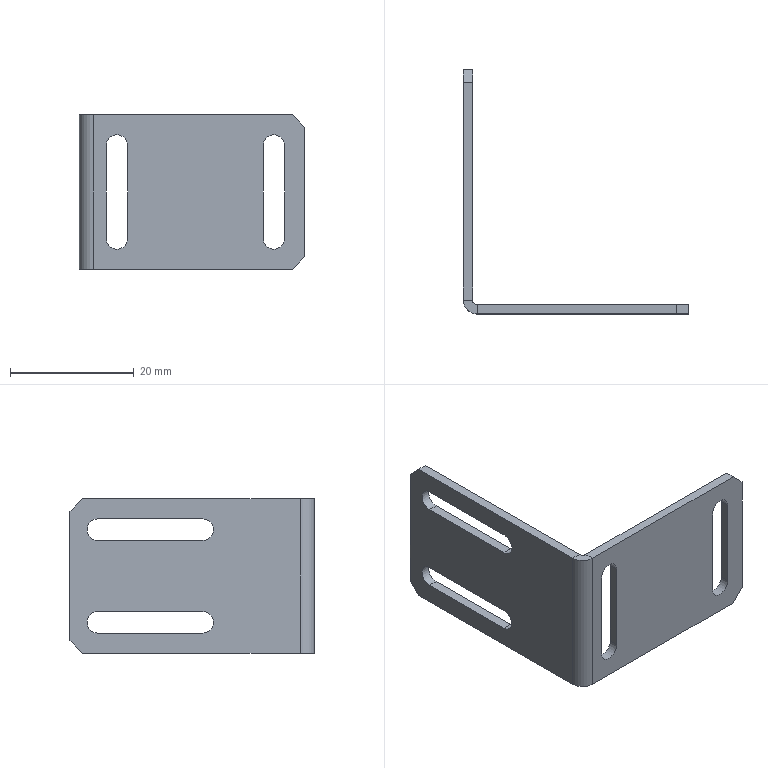Part | NX | 1 solid | 34 faces | box 36.5 x 39.5 x 25 mm | volume 2364 mm3 | plane 24 | cylinder 10 | commonest cylinder face diameters 3.5 x8 1.473 x1 4.473 x1
STEP:
#1=CARTESIAN_POINT('',(-1.5,-18.263,-12.5));
#2=VERTEX_POINT('',#1);
#3=CARTESIAN_POINT('',(-1.5,17.,-12.5));
#4=VERTEX_POINT('',#3);
#5=CARTESIAN_POINT('',(-1.5,-19.,-12.5));
#6=DIRECTION('',(0.,1.,0.));
#7=VECTOR('',#6,1000.);
#8=LINE('',#5,#7);
#9=EDGE_CURVE('',#2,#4,#8,.T.);
#10=ORIENTED_EDGE('',*,*,#9,.T.);
#11=CARTESIAN_POINT('',(0.,17.,-12.5));
#12=VERTEX_POINT('',#11);
#13=CARTESIAN_POINT('',(-1.5,17.,-12.5));
#14=DIRECTION('',(1.,0.,0.));
#15=VECTOR('',#14,1000.);
#16=LINE('',#13,#15);
#17=EDGE_CURVE('',#4,#12,#16,.T.);
#18=ORIENTED_EDGE('',*,*,#17,.T.);
#19=CARTESIAN_POINT('',(0.,-18.263,-12.5));
#20=VERTEX_POINT('',#19);
#21=CARTESIAN_POINT('',(0.,-19.,-12.5));
#22=DIRECTION('',(0.,1.,0.));
#23=VECTOR('',#22,1000.);
#24=LINE('',#21,#23);
#25=EDGE_CURVE('',#20,#12,#24,.T.);
#26=ORIENTED_EDGE('',*,*,#25,.F.);
#27=CARTESIAN_POINT('',(0.,-18.263,-12.5));
#28=DIRECTION('',(-1.,0.,0.));
#29=VECTOR('',#28,1000.);
#30=LINE('',#27,#29);
#31=EDGE_CURVE('',#20,#2,#30,.T.);
#32=ORIENTED_EDGE('',*,*,#31,.T.);
#33=EDGE_LOOP('',(#10,#18,#26,#32));
#34=FACE_BOUND('',#33,.T.);
#35=CARTESIAN_POINT('',(-1.5,-19.,-12.5));
#36=DIRECTION('',(0.,0.,-1.));
#37=DIRECTION('',(-1.,0.,0.));
#38=AXIS2_PLACEMENT_3D('',#35,#36,#37);
#39=PLANE('',#38);
#40=ADVANCED_FACE('',(#34),#39,.T.);
#41=CARTESIAN_POINT('',(-1.5,14.5,-9.25));
#42=VERTEX_POINT('',#41);
#43=CARTESIAN_POINT('',(-1.5,14.5,-5.75));
#44=VERTEX_POINT('',#43);
#45=CARTESIAN_POINT('',(-1.5,14.5,-7.5));
#46=DIRECTION('',(1.,0.,0.));
#47=DIRECTION('',(0.,0.,-1.));
#48=AXIS2_PLACEMENT_3D('',#45,#46,#47);
#49=CIRCLE('',#48,1.75);
#50=EDGE_CURVE('',#42,#44,#49,.T.);
#51=ORIENTED_EDGE('',*,*,#50,.T.);
#52=CARTESIAN_POINT('',(-1.5,-2.5,-5.75));
#53=VERTEX_POINT('',#52);
#54=CARTESIAN_POINT('',(-1.5,14.5,-5.75));
#55=DIRECTION('',(0.,-1.,0.));
#56=VECTOR('',#55,1000.);
#57=LINE('',#54,#56);
#58=EDGE_CURVE('',#44,#53,#57,.T.);
#59=ORIENTED_EDGE('',*,*,#58,.T.);
#60=CARTESIAN_POINT('',(-1.5,-2.5,-9.25));
#61=VERTEX_POINT('',#60);
#62=CARTESIAN_POINT('',(-1.5,-2.5,-7.5));
#63=DIRECTION('',(1.,0.,0.));
#64=DIRECTION('',(0.,0.,-1.));
#65=AXIS2_PLACEMENT_3D('',#62,#63,#64);
#66=CIRCLE('',#65,1.75);
#67=EDGE_CURVE('',#53,#61,#66,.T.);
#68=ORIENTED_EDGE('',*,*,#67,.T.);
#69=CARTESIAN_POINT('',(-1.5,14.5,-9.25));
#70=DIRECTION('',(0.,1.,0.));
#71=VECTOR('',#70,1000.);
#72=LINE('',#69,#71);
#73=EDGE_CURVE('',#61,#42,#72,.T.);
#74=ORIENTED_EDGE('',*,*,#73,.T.);
#75=EDGE_LOOP('',(#51,#59,#68,#74));
#76=FACE_BOUND('',#75,.T.);
#77=CARTESIAN_POINT('',(-1.5,14.5,5.75));
#78=VERTEX_POINT('',#77);
#79=CARTESIAN_POINT('',(-1.5,14.5,9.25));
#80=VERTEX_POINT('',#79);
#81=CARTESIAN_POINT('',(-1.5,14.5,7.5));
#82=DIRECTION('',(1.,0.,0.));
#83=DIRECTION('',(0.,0.,-1.));
#84=AXIS2_PLACEMENT_3D('',#81,#82,#83);
#85=CIRCLE('',#84,1.75);
#86=EDGE_CURVE('',#78,#80,#85,.T.);
#87=ORIENTED_EDGE('',*,*,#86,.T.);
#88=CARTESIAN_POINT('',(-1.5,-2.5,9.25));
#89=VERTEX_POINT('',#88);
#90=CARTESIAN_POINT('',(-1.5,14.5,9.25));
#91=DIRECTION('',(0.,-1.,0.));
#92=VECTOR('',#91,1000.);
#93=LINE('',#90,#92);
#94=EDGE_CURVE('',#80,#89,#93,.T.);
#95=ORIENTED_EDGE('',*,*,#94,.T.);
#96=CARTESIAN_POINT('',(-1.5,-2.5,5.75));
#97=VERTEX_POINT('',#96);
#98=CARTESIAN_POINT('',(-1.5,-2.5,7.5));
#99=DIRECTION('',(1.,0.,0.));
#100=DIRECTION('',(0.,0.,-1.));
#101=AXIS2_PLACEMENT_3D('',#98,#99,#100);
#102=CIRCLE('',#101,1.75);
#103=EDGE_CURVE('',#89,#97,#102,.T.);
#104=ORIENTED_EDGE('',*,*,#103,.T.);
#105=CARTESIAN_POINT('',(-1.5,14.5,5.75));
#106=DIRECTION('',(0.,1.,0.));
#107=VECTOR('',#106,1000.);
#108=LINE('',#105,#107);
#109=EDGE_CURVE('',#97,#78,#108,.T.);
#110=ORIENTED_EDGE('',*,*,#109,.T.);
#111=EDGE_LOOP('',(#87,#95,#104,#110));
#112=FACE_BOUND('',#111,.T.);
#113=CARTESIAN_POINT('',(-1.5,19.,-10.5));
#114=VERTEX_POINT('',#113);
#115=CARTESIAN_POINT('',(-1.5,19.,10.5));
#116=VERTEX_POINT('',#115);
#117=CARTESIAN_POINT('',(-1.5,19.,12.5));
#118=DIRECTION('',(0.,0.,1.));
#119=VECTOR('',#118,1000.);
#120=LINE('',#117,#119);
#121=EDGE_CURVE('',#114,#116,#120,.T.);
#122=ORIENTED_EDGE('',*,*,#121,.F.);
#123=CARTESIAN_POINT('',(-1.5,14.75,-14.75));
#124=DIRECTION('',(0.,0.7071,0.7071));
#125=VECTOR('',#124,1000.);
#126=LINE('',#123,#125);
#127=EDGE_CURVE('',#114,#4,#126,.F.);
#128=ORIENTED_EDGE('',*,*,#127,.T.);
#129=ORIENTED_EDGE('',*,*,#9,.F.);
#130=CARTESIAN_POINT('',(-1.5,-18.263,12.5));
#131=VERTEX_POINT('',#130);
#132=CARTESIAN_POINT('',(-1.5,-18.263,-12.5));
#133=DIRECTION('',(0.,0.,-1.));
#134=VECTOR('',#133,1000.);
#135=LINE('',#132,#134);
#136=EDGE_CURVE('',#2,#131,#135,.F.);
#137=ORIENTED_EDGE('',*,*,#136,.T.);
#138=CARTESIAN_POINT('',(-1.5,17.,12.5));
#139=VERTEX_POINT('',#138);
#140=CARTESIAN_POINT('',(-1.5,-19.,12.5));
#141=DIRECTION('',(0.,-1.,0.));
#142=VECTOR('',#141,1000.);
#143=LINE('',#140,#142);
#144=EDGE_CURVE('',#139,#131,#143,.T.);
#145=ORIENTED_EDGE('',*,*,#144,.F.);
#146=CARTESIAN_POINT('',(-1.5,14.75,14.75));
#147=DIRECTION('',(0.,-0.7071,0.7071));
#148=VECTOR('',#147,1000.);
#149=LINE('',#146,#148);
#150=EDGE_CURVE('',#139,#116,#149,.F.);
#151=ORIENTED_EDGE('',*,*,#150,.T.);
#152=EDGE_LOOP('',(#122,#128,#129,#137,#145,#151));
#153=FACE_BOUND('',#152,.T.);
#154=CARTESIAN_POINT('',(-1.5,0.,0.));
#155=DIRECTION('',(-1.,0.,0.));
#156=DIRECTION('',(0.,0.,1.));
#157=AXIS2_PLACEMENT_3D('',#154,#155,#156);
#158=PLANE('',#157);
#159=ADVANCED_FACE('',(#76,#112,#153),#158,.T.);
#160=CARTESIAN_POINT('',(0.,14.5,-5.75));
#161=VERTEX_POINT('',#160);
#162=CARTESIAN_POINT('',(0.,-2.5,-5.75));
#163=VERTEX_POINT('',#162);
#164=CARTESIAN_POINT('',(0.,14.5,-5.75));
#165=DIRECTION('',(0.,-1.,0.));
#166=VECTOR('',#165,1000.);
#167=LINE('',#164,#166);
#168=EDGE_CURVE('',#161,#163,#167,.T.);
#169=ORIENTED_EDGE('',*,*,#168,.F.);
#170=CARTESIAN_POINT('',(0.,14.5,-9.25));
#171=VERTEX_POINT('',#170);
#172=CARTESIAN_POINT('',(0.,14.5,-7.5));
#173=DIRECTION('',(1.,0.,0.));
#174=DIRECTION('',(0.,0.,-1.));
#175=AXIS2_PLACEMENT_3D('',#172,#173,#174);
#176=CIRCLE('',#175,1.75);
#177=EDGE_CURVE('',#171,#161,#176,.T.);
#178=ORIENTED_EDGE('',*,*,#177,.F.);
#179=CARTESIAN_POINT('',(0.,-2.5,-9.25));
#180=VERTEX_POINT('',#179);
#181=CARTESIAN_POINT('',(0.,14.5,-9.25));
#182=DIRECTION('',(0.,1.,0.));
#183=VECTOR('',#182,1000.);
#184=LINE('',#181,#183);
#185=EDGE_CURVE('',#180,#171,#184,.T.);
#186=ORIENTED_EDGE('',*,*,#185,.F.);
#187=CARTESIAN_POINT('',(0.,-2.5,-7.5));
#188=DIRECTION('',(1.,0.,0.));
#189=DIRECTION('',(0.,0.,-1.));
#190=AXIS2_PLACEMENT_3D('',#187,#188,#189);
#191=CIRCLE('',#190,1.75);
#192=EDGE_CURVE('',#163,#180,#191,.T.);
#193=ORIENTED_EDGE('',*,*,#192,.F.);
#194=EDGE_LOOP('',(#169,#178,#186,#193));
#195=FACE_BOUND('',#194,.T.);
#196=CARTESIAN_POINT('',(0.,14.5,9.25));
#197=VERTEX_POINT('',#196);
#198=CARTESIAN_POINT('',(0.,-2.5,9.25));
#199=VERTEX_POINT('',#198);
#200=CARTESIAN_POINT('',(0.,14.5,9.25));
#201=DIRECTION('',(0.,-1.,0.));
#202=VECTOR('',#201,1000.);
#203=LINE('',#200,#202);
#204=EDGE_CURVE('',#197,#199,#203,.T.);
#205=ORIENTED_EDGE('',*,*,#204,.F.);
#206=CARTESIAN_POINT('',(0.,14.5,5.75));
#207=VERTEX_POINT('',#206);
#208=CARTESIAN_POINT('',(0.,14.5,7.5));
#209=DIRECTION('',(1.,0.,0.));
#210=DIRECTION('',(0.,0.,-1.));
#211=AXIS2_PLACEMENT_3D('',#208,#209,#210);
#212=CIRCLE('',#211,1.75);
#213=EDGE_CURVE('',#207,#197,#212,.T.);
#214=ORIENTED_EDGE('',*,*,#213,.F.);
#215=CARTESIAN_POINT('',(0.,-2.5,5.75));
#216=VERTEX_POINT('',#215);
#217=CARTESIAN_POINT('',(0.,14.5,5.75));
#218=DIRECTION('',(0.,1.,0.));
#219=VECTOR('',#218,1000.);
#220=LINE('',#217,#219);
#221=EDGE_CURVE('',#216,#207,#220,.T.);
#222=ORIENTED_EDGE('',*,*,#221,.F.);
#223=CARTESIAN_POINT('',(0.,-2.5,7.5));
#224=DIRECTION('',(1.,0.,0.));
#225=DIRECTION('',(0.,0.,-1.));
#226=AXIS2_PLACEMENT_3D('',#223,#224,#225);
#227=CIRCLE('',#226,1.75);
#228=EDGE_CURVE('',#199,#216,#227,.T.);
#229=ORIENTED_EDGE('',*,*,#228,.F.);
#230=EDGE_LOOP('',(#205,#214,#222,#229));
#231=FACE_BOUND('',#230,.T.);
#232=ORIENTED_EDGE('',*,*,#25,.T.);
#233=CARTESIAN_POINT('',(0.,19.,-10.5));
#234=VERTEX_POINT('',#233);
#235=CARTESIAN_POINT('',(0.,17.,-12.5));
#236=DIRECTION('',(0.,-0.7071,-0.7071));
#237=VECTOR('',#236,1000.);
#238=LINE('',#235,#237);
#239=EDGE_CURVE('',#12,#234,#238,.F.);
#240=ORIENTED_EDGE('',*,*,#239,.T.);
#241=CARTESIAN_POINT('',(0.,19.,10.5));
#242=VERTEX_POINT('',#241);
#243=CARTESIAN_POINT('',(0.,19.,12.5));
#244=DIRECTION('',(0.,0.,1.));
#245=VECTOR('',#244,1000.);
#246=LINE('',#243,#245);
#247=EDGE_CURVE('',#234,#242,#246,.T.);
#248=ORIENTED_EDGE('',*,*,#247,.T.);
#249=CARTESIAN_POINT('',(0.,17.,12.5));
#250=VERTEX_POINT('',#249);
#251=CARTESIAN_POINT('',(0.,19.,10.5));
#252=DIRECTION('',(0.,0.7071,-0.7071));
#253=VECTOR('',#252,1000.);
#254=LINE('',#251,#253);
#255=EDGE_CURVE('',#242,#250,#254,.F.);
#256=ORIENTED_EDGE('',*,*,#255,.T.);
#257=CARTESIAN_POINT('',(0.,-18.263,12.5));
#258=VERTEX_POINT('',#257);
#259=CARTESIAN_POINT('',(0.,-19.,12.5));
#260=DIRECTION('',(0.,-1.,0.));
#261=VECTOR('',#260,1000.);
#262=LINE('',#259,#261);
#263=EDGE_CURVE('',#250,#258,#262,.T.);
#264=ORIENTED_EDGE('',*,*,#263,.T.);
#265=CARTESIAN_POINT('',(0.,-18.263,-12.5));
#266=DIRECTION('',(0.,0.,-1.));
#267=VECTOR('',#266,1000.);
#268=LINE('',#265,#267);
#269=EDGE_CURVE('',#20,#258,#268,.F.);
#270=ORIENTED_EDGE('',*,*,#269,.F.);
#271=EDGE_LOOP('',(#232,#240,#248,#256,#264,#270));
#272=FACE_BOUND('',#271,.T.);
#273=CARTESIAN_POINT('',(0.,0.,0.));
#274=DIRECTION('',(-1.,0.,0.));
#275=DIRECTION('',(0.,0.,1.));
#276=AXIS2_PLACEMENT_3D('',#273,#274,#275);
#277=PLANE('',#276);
#278=ADVANCED_FACE('',(#195,#231,#272),#277,.F.);
#279=ORIENTED_EDGE('',*,*,#263,.F.);
#280=CARTESIAN_POINT('',(-1.5,17.,12.5));
#281=DIRECTION('',(-1.,0.,0.));
#282=VECTOR('',#281,1000.);
#283=LINE('',#280,#282);
#284=EDGE_CURVE('',#250,#139,#283,.T.);
#285=ORIENTED_EDGE('',*,*,#284,.T.);
#286=ORIENTED_EDGE('',*,*,#144,.T.);
#287=CARTESIAN_POINT('',(0.,-18.263,12.5));
#288=DIRECTION('',(-1.,0.,0.));
#289=VECTOR('',#288,1000.);
#290=LINE('',#287,#289);
#291=EDGE_CURVE('',#258,#131,#290,.T.);
#292=ORIENTED_EDGE('',*,*,#291,.F.);
#293=EDGE_LOOP('',(#279,#285,#286,#292));
#294=FACE_BOUND('',#293,.T.);
#295=CARTESIAN_POINT('',(-1.5,-19.,12.5));
#296=DIRECTION('',(0.,0.,1.));
#297=DIRECTION('',(1.,0.,0.));
#298=AXIS2_PLACEMENT_3D('',#295,#296,#297);
#299=PLANE('',#298);
#300=ADVANCED_FACE('',(#294),#299,.T.);
#301=ORIENTED_EDGE('',*,*,#247,.F.);
#302=CARTESIAN_POINT('',(-1.5,19.,-10.5));
#303=DIRECTION('',(-1.,0.,0.));
#304=VECTOR('',#303,1000.);
#305=LINE('',#302,#304);
#306=EDGE_CURVE('',#234,#114,#305,.T.);
#307=ORIENTED_EDGE('',*,*,#306,.T.);
#308=ORIENTED_EDGE('',*,*,#121,.T.);
#309=CARTESIAN_POINT('',(-1.5,19.,10.5));
#310=DIRECTION('',(1.,0.,0.));
#311=VECTOR('',#310,1000.);
#312=LINE('',#309,#311);
#313=EDGE_CURVE('',#116,#242,#312,.T.);
#314=ORIENTED_EDGE('',*,*,#313,.T.);
#315=EDGE_LOOP('',(#301,#307,#308,#314));
#316=FACE_BOUND('',#315,.T.);
#317=CARTESIAN_POINT('',(-1.5,19.,12.5));
#318=DIRECTION('',(0.,1.,0.));
#319=DIRECTION('',(0.,0.,1.));
#320=AXIS2_PLACEMENT_3D('',#317,#318,#319);
#321=PLANE('',#320);
#322=ADVANCED_FACE('',(#316),#321,.T.);
#323=CARTESIAN_POINT('',(0.7366,-19.,12.5));
#324=VERTEX_POINT('',#323);
#325=CARTESIAN_POINT('',(0.7366,-20.5,12.5));
#326=VERTEX_POINT('',#325);
#327=CARTESIAN_POINT('',(0.7366,-19.,12.5));
#328=DIRECTION('',(0.,-1.,0.));
#329=VECTOR('',#328,1000.);
#330=LINE('',#327,#329);
#331=EDGE_CURVE('',#324,#326,#330,.T.);
#332=ORIENTED_EDGE('',*,*,#331,.F.);
#333=CARTESIAN_POINT('',(0.7366,-18.263,12.5));
#334=DIRECTION('',(0.,0.,-1.));
#335=DIRECTION('',(-1.,0.,0.));
#336=AXIS2_PLACEMENT_3D('',#333,#334,#335);
#337=CIRCLE('',#336,0.7366);
#338=EDGE_CURVE('',#258,#324,#337,.F.);
#339=ORIENTED_EDGE('',*,*,#338,.F.);
#340=ORIENTED_EDGE('',*,*,#291,.T.);
#341=CARTESIAN_POINT('',(0.7366,-18.263,12.5));
#342=DIRECTION('',(0.,0.,-1.));
#343=DIRECTION('',(-1.,0.,0.));
#344=AXIS2_PLACEMENT_3D('',#341,#342,#343);
#345=CIRCLE('',#344,2.237);
#346=EDGE_CURVE('',#131,#326,#345,.F.);
#347=ORIENTED_EDGE('',*,*,#346,.T.);
#348=EDGE_LOOP('',(#332,#339,#340,#347));
#349=FACE_BOUND('',#348,.T.);
#350=CARTESIAN_POINT('',(0.7366,-18.263,12.5));
#351=DIRECTION('',(0.,0.,1.));
#352=DIRECTION('',(1.,0.,0.));
#353=AXIS2_PLACEMENT_3D('',#350,#351,#352);
#354=PLANE('',#353);
#355=ADVANCED_FACE('',(#349),#354,.T.);
#356=CARTESIAN_POINT('',(0.7366,-19.,-12.5));
#357=VERTEX_POINT('',#356);
#358=CARTESIAN_POINT('',(0.7366,-18.263,-12.5));
#359=DIRECTION('',(0.,0.,-1.));
#360=DIRECTION('',(-1.,0.,0.));
#361=AXIS2_PLACEMENT_3D('',#358,#359,#360);
#362=CIRCLE('',#361,0.7366);
#363=EDGE_CURVE('',#357,#20,#362,.T.);
#364=ORIENTED_EDGE('',*,*,#363,.F.);
#365=CARTESIAN_POINT('',(0.7366,-20.5,-12.5));
#366=VERTEX_POINT('',#365);
#367=CARTESIAN_POINT('',(0.7366,-19.,-12.5));
#368=DIRECTION('',(0.,-1.,0.));
#369=VECTOR('',#368,1000.);
#370=LINE('',#367,#369);
#371=EDGE_CURVE('',#357,#366,#370,.T.);
#372=ORIENTED_EDGE('',*,*,#371,.T.);
#373=CARTESIAN_POINT('',(0.7366,-18.263,-12.5));
#374=DIRECTION('',(0.,0.,-1.));
#375=DIRECTION('',(-1.,0.,0.));
#376=AXIS2_PLACEMENT_3D('',#373,#374,#375);
#377=CIRCLE('',#376,2.237);
#378=EDGE_CURVE('',#366,#2,#377,.T.);
#379=ORIENTED_EDGE('',*,*,#378,.T.);
#380=ORIENTED_EDGE('',*,*,#31,.F.);
#381=EDGE_LOOP('',(#364,#372,#379,#380));
#382=FACE_BOUND('',#381,.T.);
#383=CARTESIAN_POINT('',(0.7366,-18.263,-12.5));
#384=DIRECTION('',(0.,0.,1.));
#385=DIRECTION('',(1.,0.,0.));
#386=AXIS2_PLACEMENT_3D('',#383,#384,#385);
#387=PLANE('',#386);
#388=ADVANCED_FACE('',(#382),#387,.F.);
#389=ORIENTED_EDGE('',*,*,#136,.F.);
#390=ORIENTED_EDGE('',*,*,#378,.F.);
#391=CARTESIAN_POINT('',(0.7366,-20.5,0.));
#392=DIRECTION('',(0.,0.,1.));
#393=VECTOR('',#392,1000.);
#394=LINE('',#391,#393);
#395=EDGE_CURVE('',#366,#326,#394,.T.);
#396=ORIENTED_EDGE('',*,*,#395,.T.);
#397=ORIENTED_EDGE('',*,*,#346,.F.);
#398=EDGE_LOOP('',(#389,#390,#396,#397));
#399=FACE_BOUND('',#398,.T.);
#400=CARTESIAN_POINT('',(0.7366,-18.263,-12.5));
#401=DIRECTION('',(0.,0.,-1.));
#402=DIRECTION('',(0.,-1.,0.));
#403=AXIS2_PLACEMENT_3D('',#400,#401,#402);
#404=CYLINDRICAL_SURFACE('',#403,2.237);
#405=ADVANCED_FACE('',(#399),#404,.T.);
#406=ORIENTED_EDGE('',*,*,#269,.T.);
#407=ORIENTED_EDGE('',*,*,#338,.T.);
#408=CARTESIAN_POINT('',(0.7366,-19.,12.5));
#409=DIRECTION('',(0.,0.,-1.));
#410=VECTOR('',#409,1000.);
#411=LINE('',#408,#410);
#412=EDGE_CURVE('',#324,#357,#411,.T.);
#413=ORIENTED_EDGE('',*,*,#412,.T.);
#414=ORIENTED_EDGE('',*,*,#363,.T.);
#415=EDGE_LOOP('',(#406,#407,#413,#414));
#416=FACE_BOUND('',#415,.T.);
#417=CARTESIAN_POINT('',(0.7366,-18.263,-12.5));
#418=DIRECTION('',(0.,0.,-1.));
#419=DIRECTION('',(0.,-1.,0.));
#420=AXIS2_PLACEMENT_3D('',#417,#418,#419);
#421=CYLINDRICAL_SURFACE('',#420,0.7366);
#422=ADVANCED_FACE('',(#416),#421,.F.);
#423=CARTESIAN_POINT('',(33.,-20.5,12.5));
#424=VERTEX_POINT('',#423);
#425=CARTESIAN_POINT('',(0.,-20.5,12.5));
#426=DIRECTION('',(-1.,0.,0.));
#427=VECTOR('',#426,1000.);
#428=LINE('',#425,#427);
#429=EDGE_CURVE('',#424,#326,#428,.T.);
#430=ORIENTED_EDGE('',*,*,#429,.F.);
#431=CARTESIAN_POINT('',(33.,-19.,12.5));
#432=VERTEX_POINT('',#431);
#433=CARTESIAN_POINT('',(33.,-20.5,12.5));
#434=DIRECTION('',(0.,1.,0.));
#435=VECTOR('',#434,1000.);
#436=LINE('',#433,#435);
#437=EDGE_CURVE('',#424,#432,#436,.T.);
#438=ORIENTED_EDGE('',*,*,#437,.T.);
#439=CARTESIAN_POINT('',(0.,-19.,12.5));
#440=DIRECTION('',(-1.,0.,0.));
#441=VECTOR('',#440,1000.);
#442=LINE('',#439,#441);
#443=EDGE_CURVE('',#432,#324,#442,.T.);
#444=ORIENTED_EDGE('',*,*,#443,.T.);
#445=ORIENTED_EDGE('',*,*,#331,.T.);
#446=EDGE_LOOP('',(#430,#438,#444,#445));
#447=FACE_BOUND('',#446,.T.);
#448=CARTESIAN_POINT('',(0.,-20.5,12.5));
#449=DIRECTION('',(0.,0.,-1.));
#450=DIRECTION('',(-1.,0.,0.));
#451=AXIS2_PLACEMENT_3D('',#448,#449,#450);
#452=PLANE('',#451);
#453=ADVANCED_FACE('',(#447),#452,.F.);
#454=CARTESIAN_POINT('',(33.,-19.,-12.5));
#455=VERTEX_POINT('',#454);
#456=CARTESIAN_POINT('',(35.,-19.,-12.5));
#457=DIRECTION('',(1.,0.,0.));
#458=VECTOR('',#457,1000.);
#459=LINE('',#456,#458);
#460=EDGE_CURVE('',#357,#455,#459,.T.);
#461=ORIENTED_EDGE('',*,*,#460,.T.);
#462=CARTESIAN_POINT('',(33.,-20.5,-12.5));
#463=VERTEX_POINT('',#462);
#464=CARTESIAN_POINT('',(33.,-20.5,-12.5));
#465=DIRECTION('',(0.,-1.,0.));
#466=VECTOR('',#465,1000.);
#467=LINE('',#464,#466);
#468=EDGE_CURVE('',#455,#463,#467,.T.);
#469=ORIENTED_EDGE('',*,*,#468,.T.);
#470=CARTESIAN_POINT('',(35.,-20.5,-12.5));
#471=DIRECTION('',(1.,0.,0.));
#472=VECTOR('',#471,1000.);
#473=LINE('',#470,#472);
#474=EDGE_CURVE('',#366,#463,#473,.T.);
#475=ORIENTED_EDGE('',*,*,#474,.F.);
#476=ORIENTED_EDGE('',*,*,#371,.F.);
#477=EDGE_LOOP('',(#461,#469,#475,#476));
#478=FACE_BOUND('',#477,.T.);
#479=CARTESIAN_POINT('',(35.,-20.5,-12.5));
#480=DIRECTION('',(0.,0.,1.));
#481=DIRECTION('',(1.,0.,0.));
#482=AXIS2_PLACEMENT_3D('',#479,#480,#481);
#483=PLANE('',#482);
#484=ADVANCED_FACE('',(#478),#483,.F.);
#485=CARTESIAN_POINT('',(2.85,-20.5,7.5));
#486=VERTEX_POINT('',#485);
#487=CARTESIAN_POINT('',(2.85,-20.5,-7.5));
#488=VERTEX_POINT('',#487);
#489=CARTESIAN_POINT('',(2.85,-20.5,7.5));
#490=DIRECTION('',(0.,0.,-1.));
#491=VECTOR('',#490,1000.);
#492=LINE('',#489,#491);
#493=EDGE_CURVE('',#486,#488,#492,.T.);
#494=ORIENTED_EDGE('',*,*,#493,.F.);
#495=CARTESIAN_POINT('',(6.35,-20.5,7.5));
#496=VERTEX_POINT('',#495);
#497=CARTESIAN_POINT('',(4.6,-20.5,7.5));
#498=DIRECTION('',(0.,-1.,0.));
#499=DIRECTION('',(1.,0.,0.));
#500=AXIS2_PLACEMENT_3D('',#497,#498,#499);
#501=CIRCLE('',#500,1.75);
#502=EDGE_CURVE('',#496,#486,#501,.T.);
#503=ORIENTED_EDGE('',*,*,#502,.F.);
#504=CARTESIAN_POINT('',(6.35,-20.5,-7.5));
#505=VERTEX_POINT('',#504);
#506=CARTESIAN_POINT('',(6.35,-20.5,7.5));
#507=DIRECTION('',(0.,0.,1.));
#508=VECTOR('',#507,1000.);
#509=LINE('',#506,#508);
#510=EDGE_CURVE('',#505,#496,#509,.T.);
#511=ORIENTED_EDGE('',*,*,#510,.F.);
#512=CARTESIAN_POINT('',(4.6,-20.5,-7.5));
#513=DIRECTION('',(0.,-1.,0.));
#514=DIRECTION('',(1.,0.,0.));
#515=AXIS2_PLACEMENT_3D('',#512,#513,#514);
#516=CIRCLE('',#515,1.75);
#517=EDGE_CURVE('',#488,#505,#516,.T.);
#518=ORIENTED_EDGE('',*,*,#517,.F.);
#519=EDGE_LOOP('',(#494,#503,#511,#518));
#520=FACE_BOUND('',#519,.T.);
#521=CARTESIAN_POINT('',(28.25,-20.5,7.5));
#522=VERTEX_POINT('',#521);
#523=CARTESIAN_POINT('',(28.25,-20.5,-7.5));
#524=VERTEX_POINT('',#523);
#525=CARTESIAN_POINT('',(28.25,-20.5,7.5));
#526=DIRECTION('',(0.,0.,-1.));
#527=VECTOR('',#526,1000.);
#528=LINE('',#525,#527);
#529=EDGE_CURVE('',#522,#524,#528,.T.);
#530=ORIENTED_EDGE('',*,*,#529,.F.);
#531=CARTESIAN_POINT('',(31.75,-20.5,7.5));
#532=VERTEX_POINT('',#531);
#533=CARTESIAN_POINT('',(30.,-20.5,7.5));
#534=DIRECTION('',(0.,-1.,0.));
#535=DIRECTION('',(1.,0.,0.));
#536=AXIS2_PLACEMENT_3D('',#533,#534,#535);
#537=CIRCLE('',#536,1.75);
#538=EDGE_CURVE('',#532,#522,#537,.T.);
#539=ORIENTED_EDGE('',*,*,#538,.F.);
#540=CARTESIAN_POINT('',(31.75,-20.5,-7.5));
#541=VERTEX_POINT('',#540);
#542=CARTESIAN_POINT('',(31.75,-20.5,7.5));
#543=DIRECTION('',(0.,0.,1.));
#544=VECTOR('',#543,1000.);
#545=LINE('',#542,#544);
#546=EDGE_CURVE('',#541,#532,#545,.T.);
#547=ORIENTED_EDGE('',*,*,#546,.F.);
#548=CARTESIAN_POINT('',(30.,-20.5,-7.5));
#549=DIRECTION('',(0.,-1.,0.));
#550=DIRECTION('',(1.,0.,0.));
#551=AXIS2_PLACEMENT_3D('',#548,#549,#550);
#552=CIRCLE('',#551,1.75);
#553=EDGE_CURVE('',#524,#541,#552,.T.);
#554=ORIENTED_EDGE('',*,*,#553,.F.);
#555=EDGE_LOOP('',(#530,#539,#547,#554));
#556=FACE_BOUND('',#555,.T.);
#557=ORIENTED_EDGE('',*,*,#474,.T.);
#558=CARTESIAN_POINT('',(35.,-20.5,-10.5));
#559=VERTEX_POINT('',#558);
#560=CARTESIAN_POINT('',(35.,-20.5,-10.5));
#561=DIRECTION('',(-0.7071,0.,-0.7071));
#562=VECTOR('',#561,1000.);
#563=LINE('',#560,#562);
#564=EDGE_CURVE('',#463,#559,#563,.F.);
#565=ORIENTED_EDGE('',*,*,#564,.T.);
#566=CARTESIAN_POINT('',(35.,-20.5,10.5));
#567=VERTEX_POINT('',#566);
#568=CARTESIAN_POINT('',(35.,-20.5,12.5));
#569=DIRECTION('',(0.,0.,1.));
#570=VECTOR('',#569,1000.);
#571=LINE('',#568,#570);
#572=EDGE_CURVE('',#559,#567,#571,.T.);
#573=ORIENTED_EDGE('',*,*,#572,.T.);
#574=CARTESIAN_POINT('',(33.,-20.5,12.5));
#575=DIRECTION('',(0.7071,0.,-0.7071));
#576=VECTOR('',#575,1000.);
#577=LINE('',#574,#576);
#578=EDGE_CURVE('',#567,#424,#577,.F.);
#579=ORIENTED_EDGE('',*,*,#578,.T.);
#580=ORIENTED_EDGE('',*,*,#429,.T.);
#581=ORIENTED_EDGE('',*,*,#395,.F.);
#582=EDGE_LOOP('',(#557,#565,#573,#579,#580,#581));
#583=FACE_BOUND('',#582,.T.);
#584=CARTESIAN_POINT('',(0.,-20.5,0.));
#585=DIRECTION('',(0.,1.,0.));
#586=DIRECTION('',(-1.,0.,0.));
#587=AXIS2_PLACEMENT_3D('',#584,#585,#586);
#588=PLANE('',#587);
#589=ADVANCED_FACE('',(#520,#556,#583),#588,.F.);
#590=CARTESIAN_POINT('',(2.85,-19.,7.5));
#591=VERTEX_POINT('',#590);
#592=CARTESIAN_POINT('',(6.35,-19.,7.5));
#593=VERTEX_POINT('',#592);
#594=CARTESIAN_POINT('',(4.6,-19.,7.5));
#595=DIRECTION('',(0.,1.,0.));
#596=DIRECTION('',(-1.,0.,0.));
#597=AXIS2_PLACEMENT_3D('',#594,#595,#596);
#598=CIRCLE('',#597,1.75);
#599=EDGE_CURVE('',#591,#593,#598,.T.);
#600=ORIENTED_EDGE('',*,*,#599,.F.);
#601=CARTESIAN_POINT('',(2.85,-19.,-7.5));
#602=VERTEX_POINT('',#601);
#603=CARTESIAN_POINT('',(2.85,-19.,0.));
#604=DIRECTION('',(0.,0.,1.));
#605=VECTOR('',#604,1000.);
#606=LINE('',#603,#605);
#607=EDGE_CURVE('',#602,#591,#606,.T.);
#608=ORIENTED_EDGE('',*,*,#607,.F.);
#609=CARTESIAN_POINT('',(6.35,-19.,-7.5));
#610=VERTEX_POINT('',#609);
#611=CARTESIAN_POINT('',(4.6,-19.,-7.5));
#612=DIRECTION('',(0.,1.,0.));
#613=DIRECTION('',(-1.,0.,0.));
#614=AXIS2_PLACEMENT_3D('',#611,#612,#613);
#615=CIRCLE('',#614,1.75);
#616=EDGE_CURVE('',#610,#602,#615,.T.);
#617=ORIENTED_EDGE('',*,*,#616,.F.);
#618=CARTESIAN_POINT('',(6.35,-19.,0.));
#619=DIRECTION('',(0.,0.,-1.));
#620=VECTOR('',#619,1000.);
#621=LINE('',#618,#620);
#622=EDGE_CURVE('',#593,#610,#621,.T.);
#623=ORIENTED_EDGE('',*,*,#622,.F.);
#624=EDGE_LOOP('',(#600,#608,#617,#623));
#625=FACE_BOUND('',#624,.T.);
#626=CARTESIAN_POINT('',(28.25,-19.,7.5));
#627=VERTEX_POINT('',#626);
#628=CARTESIAN_POINT('',(31.75,-19.,7.5));
#629=VERTEX_POINT('',#628);
#630=CARTESIAN_POINT('',(30.,-19.,7.5));
#631=DIRECTION('',(0.,1.,0.));
#632=DIRECTION('',(-1.,0.,0.));
#633=AXIS2_PLACEMENT_3D('',#630,#631,#632);
#634=CIRCLE('',#633,1.75);
#635=EDGE_CURVE('',#627,#629,#634,.T.);
#636=ORIENTED_EDGE('',*,*,#635,.F.);
#637=CARTESIAN_POINT('',(28.25,-19.,-7.5));
#638=VERTEX_POINT('',#637);
#639=CARTESIAN_POINT('',(28.25,-19.,0.));
#640=DIRECTION('',(0.,0.,1.));
#641=VECTOR('',#640,1000.);
#642=LINE('',#639,#641);
#643=EDGE_CURVE('',#638,#627,#642,.T.);
#644=ORIENTED_EDGE('',*,*,#643,.F.);
#645=CARTESIAN_POINT('',(31.75,-19.,-7.5));
#646=VERTEX_POINT('',#645);
#647=CARTESIAN_POINT('',(30.,-19.,-7.5));
#648=DIRECTION('',(0.,1.,0.));
#649=DIRECTION('',(-1.,0.,0.));
#650=AXIS2_PLACEMENT_3D('',#647,#648,#649);
#651=CIRCLE('',#650,1.75);
#652=EDGE_CURVE('',#646,#638,#651,.T.);
#653=ORIENTED_EDGE('',*,*,#652,.F.);
#654=CARTESIAN_POINT('',(31.75,-19.,0.));
#655=DIRECTION('',(0.,0.,-1.));
#656=VECTOR('',#655,1000.);
#657=LINE('',#654,#656);
#658=EDGE_CURVE('',#629,#646,#657,.T.);
#659=ORIENTED_EDGE('',*,*,#658,.F.);
#660=EDGE_LOOP('',(#636,#644,#653,#659));
#661=FACE_BOUND('',#660,.T.);
#662=CARTESIAN_POINT('',(35.,-19.,-10.5));
#663=VERTEX_POINT('',#662);
#664=CARTESIAN_POINT('',(35.,-19.,10.5));
#665=VERTEX_POINT('',#664);
#666=CARTESIAN_POINT('',(35.,-19.,12.5));
#667=DIRECTION('',(0.,0.,1.));
#668=VECTOR('',#667,1000.);
#669=LINE('',#666,#668);
#670=EDGE_CURVE('',#663,#665,#669,.T.);
#671=ORIENTED_EDGE('',*,*,#670,.F.);
#672=CARTESIAN_POINT('',(22.75,-19.,-22.75));
#673=DIRECTION('',(0.7071,0.,0.7071));
#674=VECTOR('',#673,1000.);
#675=LINE('',#672,#674);
#676=EDGE_CURVE('',#663,#455,#675,.F.);
#677=ORIENTED_EDGE('',*,*,#676,.T.);
#678=ORIENTED_EDGE('',*,*,#460,.F.);
#679=ORIENTED_EDGE('',*,*,#412,.F.);
#680=ORIENTED_EDGE('',*,*,#443,.F.);
#681=CARTESIAN_POINT('',(22.75,-19.,22.75));
#682=DIRECTION('',(-0.7071,0.,0.7071));
#683=VECTOR('',#682,1000.);
#684=LINE('',#681,#683);
#685=EDGE_CURVE('',#432,#665,#684,.F.);
#686=ORIENTED_EDGE('',*,*,#685,.T.);
#687=EDGE_LOOP('',(#671,#677,#678,#679,#680,#686));
#688=FACE_BOUND('',#687,.T.);
#689=CARTESIAN_POINT('',(0.,-19.,0.));
#690=DIRECTION('',(0.,1.,0.));
#691=DIRECTION('',(-1.,0.,0.));
#692=AXIS2_PLACEMENT_3D('',#689,#690,#691);
#693=PLANE('',#692);
#694=ADVANCED_FACE('',(#625,#661,#688),#693,.T.);
#695=ORIENTED_EDGE('',*,*,#572,.F.);
#696=CARTESIAN_POINT('',(35.,-20.5,-10.5));
#697=DIRECTION('',(0.,1.,0.));
#698=VECTOR('',#697,1000.);
#699=LINE('',#696,#698);
#700=EDGE_CURVE('',#559,#663,#699,.T.);
#701=ORIENTED_EDGE('',*,*,#700,.T.);
#702=ORIENTED_EDGE('',*,*,#670,.T.);
#703=CARTESIAN_POINT('',(35.,-20.5,10.5));
#704=DIRECTION('',(0.,-1.,0.));
#705=VECTOR('',#704,1000.);
#706=LINE('',#703,#705);
#707=EDGE_CURVE('',#665,#567,#706,.T.);
#708=ORIENTED_EDGE('',*,*,#707,.T.);
#709=EDGE_LOOP('',(#695,#701,#702,#708));
#710=FACE_BOUND('',#709,.T.);
#711=CARTESIAN_POINT('',(35.,-20.5,12.5));
#712=DIRECTION('',(-1.,0.,0.));
#713=DIRECTION('',(0.,-1.,0.));
#714=AXIS2_PLACEMENT_3D('',#711,#712,#713);
#715=PLANE('',#714);
#716=ADVANCED_FACE('',(#710),#715,.F.);
#717=ORIENTED_EDGE('',*,*,#213,.T.);
#718=CARTESIAN_POINT('',(-1.5,14.5,9.25));
#719=DIRECTION('',(1.,0.,0.));
#720=VECTOR('',#719,1000.);
#721=LINE('',#718,#720);
#722=EDGE_CURVE('',#80,#197,#721,.T.);
#723=ORIENTED_EDGE('',*,*,#722,.F.);
#724=ORIENTED_EDGE('',*,*,#86,.F.);
#725=CARTESIAN_POINT('',(-1.5,14.5,5.75));
#726=DIRECTION('',(1.,0.,0.));
#727=VECTOR('',#726,1000.);
#728=LINE('',#725,#727);
#729=EDGE_CURVE('',#78,#207,#728,.T.);
#730=ORIENTED_EDGE('',*,*,#729,.T.);
#731=EDGE_LOOP('',(#717,#723,#724,#730));
#732=FACE_BOUND('',#731,.T.);
#733=CARTESIAN_POINT('',(-1.5,14.5,7.5));
#734=DIRECTION('',(1.,0.,0.));
#735=DIRECTION('',(0.,0.,-1.));
#736=AXIS2_PLACEMENT_3D('',#733,#734,#735);
#737=CYLINDRICAL_SURFACE('',#736,1.75);
#738=ADVANCED_FACE('',(#732),#737,.F.);
#739=ORIENTED_EDGE('',*,*,#221,.T.);
#740=ORIENTED_EDGE('',*,*,#729,.F.);
#741=ORIENTED_EDGE('',*,*,#109,.F.);
#742=CARTESIAN_POINT('',(-1.5,-2.5,5.75));
#743=DIRECTION('',(1.,0.,0.));
#744=VECTOR('',#743,1000.);
#745=LINE('',#742,#744);
#746=EDGE_CURVE('',#97,#216,#745,.T.);
#747=ORIENTED_EDGE('',*,*,#746,.T.);
#748=EDGE_LOOP('',(#739,#740,#741,#747));
#749=FACE_BOUND('',#748,.T.);
#750=CARTESIAN_POINT('',(-1.5,14.5,5.75));
#751=DIRECTION('',(0.,0.,-1.));
#752=DIRECTION('',(0.,1.,0.));
#753=AXIS2_PLACEMENT_3D('',#750,#751,#752);
#754=PLANE('',#753);
#755=ADVANCED_FACE('',(#749),#754,.F.);
#756=ORIENTED_EDGE('',*,*,#228,.T.);
#757=ORIENTED_EDGE('',*,*,#746,.F.);
#758=ORIENTED_EDGE('',*,*,#103,.F.);
#759=CARTESIAN_POINT('',(-1.5,-2.5,9.25));
#760=DIRECTION('',(1.,0.,0.));
#761=VECTOR('',#760,1000.);
#762=LINE('',#759,#761);
#763=EDGE_CURVE('',#89,#199,#762,.T.);
#764=ORIENTED_EDGE('',*,*,#763,.T.);
#765=EDGE_LOOP('',(#756,#757,#758,#764));
#766=FACE_BOUND('',#765,.T.);
#767=CARTESIAN_POINT('',(-1.5,-2.5,7.5));
#768=DIRECTION('',(1.,0.,0.));
#769=DIRECTION('',(0.,0.,-1.));
#770=AXIS2_PLACEMENT_3D('',#767,#768,#769);
#771=CYLINDRICAL_SURFACE('',#770,1.75);
#772=ADVANCED_FACE('',(#766),#771,.F.);
#773=ORIENTED_EDGE('',*,*,#204,.T.);
#774=ORIENTED_EDGE('',*,*,#763,.F.);
#775=ORIENTED_EDGE('',*,*,#94,.F.);
#776=ORIENTED_EDGE('',*,*,#722,.T.);
#777=EDGE_LOOP('',(#773,#774,#775,#776));
#778=FACE_BOUND('',#777,.T.);
#779=CARTESIAN_POINT('',(-1.5,14.5,9.25));
#780=DIRECTION('',(0.,0.,1.));
#781=DIRECTION('',(0.,-1.,0.));
#782=AXIS2_PLACEMENT_3D('',#779,#780,#781);
#783=PLANE('',#782);
#784=ADVANCED_FACE('',(#778),#783,.F.);
#785=ORIENTED_EDGE('',*,*,#177,.T.);
#786=CARTESIAN_POINT('',(-1.5,14.5,-5.75));
#787=DIRECTION('',(1.,0.,0.));
#788=VECTOR('',#787,1000.);
#789=LINE('',#786,#788);
#790=EDGE_CURVE('',#44,#161,#789,.T.);
#791=ORIENTED_EDGE('',*,*,#790,.F.);
#792=ORIENTED_EDGE('',*,*,#50,.F.);
#793=CARTESIAN_POINT('',(-1.5,14.5,-9.25));
#794=DIRECTION('',(1.,0.,0.));
#795=VECTOR('',#794,1000.);
#796=LINE('',#793,#795);
#797=EDGE_CURVE('',#42,#171,#796,.T.);
#798=ORIENTED_EDGE('',*,*,#797,.T.);
#799=EDGE_LOOP('',(#785,#791,#792,#798));
#800=FACE_BOUND('',#799,.T.);
#801=CARTESIAN_POINT('',(-1.5,14.5,-7.5));
#802=DIRECTION('',(1.,0.,0.));
#803=DIRECTION('',(0.,0.,-1.));
#804=AXIS2_PLACEMENT_3D('',#801,#802,#803);
#805=CYLINDRICAL_SURFACE('',#804,1.75);
#806=ADVANCED_FACE('',(#800),#805,.F.);
#807=ORIENTED_EDGE('',*,*,#185,.T.);
#808=ORIENTED_EDGE('',*,*,#797,.F.);
#809=ORIENTED_EDGE('',*,*,#73,.F.);
#810=CARTESIAN_POINT('',(-1.5,-2.5,-9.25));
#811=DIRECTION('',(1.,0.,0.));
#812=VECTOR('',#811,1000.);
#813=LINE('',#810,#812);
#814=EDGE_CURVE('',#61,#180,#813,.T.);
#815=ORIENTED_EDGE('',*,*,#814,.T.);
#816=EDGE_LOOP('',(#807,#808,#809,#815));
#817=FACE_BOUND('',#816,.T.);
#818=CARTESIAN_POINT('',(-1.5,14.5,-9.25));
#819=DIRECTION('',(0.,0.,-1.));
#820=DIRECTION('',(0.,1.,0.));
#821=AXIS2_PLACEMENT_3D('',#818,#819,#820);
#822=PLANE('',#821);
#823=ADVANCED_FACE('',(#817),#822,.F.);
#824=ORIENTED_EDGE('',*,*,#192,.T.);
#825=ORIENTED_EDGE('',*,*,#814,.F.);
#826=ORIENTED_EDGE('',*,*,#67,.F.);
#827=CARTESIAN_POINT('',(-1.5,-2.5,-5.75));
#828=DIRECTION('',(1.,0.,0.));
#829=VECTOR('',#828,1000.);
#830=LINE('',#827,#829);
#831=EDGE_CURVE('',#53,#163,#830,.T.);
#832=ORIENTED_EDGE('',*,*,#831,.T.);
#833=EDGE_LOOP('',(#824,#825,#826,#832));
#834=FACE_BOUND('',#833,.T.);
#835=CARTESIAN_POINT('',(-1.5,-2.5,-7.5));
#836=DIRECTION('',(1.,0.,0.));
#837=DIRECTION('',(0.,0.,-1.));
#838=AXIS2_PLACEMENT_3D('',#835,#836,#837);
#839=CYLINDRICAL_SURFACE('',#838,1.75);
#840=ADVANCED_FACE('',(#834),#839,.F.);
#841=ORIENTED_EDGE('',*,*,#168,.T.);
#842=ORIENTED_EDGE('',*,*,#831,.F.);
#843=ORIENTED_EDGE('',*,*,#58,.F.);
#844=ORIENTED_EDGE('',*,*,#790,.T.);
#845=EDGE_LOOP('',(#841,#842,#843,#844));
#846=FACE_BOUND('',#845,.T.);
#847=CARTESIAN_POINT('',(-1.5,14.5,-5.75));
#848=DIRECTION('',(0.,0.,1.));
#849=DIRECTION('',(0.,-1.,0.));
#850=AXIS2_PLACEMENT_3D('',#847,#848,#849);
#851=PLANE('',#850);
#852=ADVANCED_FACE('',(#846),#851,.F.);
#853=ORIENTED_EDGE('',*,*,#564,.F.);
#854=ORIENTED_EDGE('',*,*,#468,.F.);
#855=ORIENTED_EDGE('',*,*,#676,.F.);
#856=ORIENTED_EDGE('',*,*,#700,.F.);
#857=EDGE_LOOP('',(#853,#854,#855,#856));
#858=FACE_BOUND('',#857,.T.);
#859=CARTESIAN_POINT('',(35.,-20.5,-10.5));
#860=DIRECTION('',(-0.7071,0.,0.7071));
#861=DIRECTION('',(0.,1.,0.));
#862=AXIS2_PLACEMENT_3D('',#859,#860,#861);
#863=PLANE('',#862);
#864=ADVANCED_FACE('',(#858),#863,.F.);
#865=ORIENTED_EDGE('',*,*,#578,.F.);
#866=ORIENTED_EDGE('',*,*,#707,.F.);
#867=ORIENTED_EDGE('',*,*,#685,.F.);
#868=ORIENTED_EDGE('',*,*,#437,.F.);
#869=EDGE_LOOP('',(#865,#866,#867,#868));
#870=FACE_BOUND('',#869,.T.);
#871=CARTESIAN_POINT('',(33.,-20.5,12.5));
#872=DIRECTION('',(-0.7071,0.,-0.7071));
#873=DIRECTION('',(0.,1.,0.));
#874=AXIS2_PLACEMENT_3D('',#871,#872,#873);
#875=PLANE('',#874);
#876=ADVANCED_FACE('',(#870),#875,.F.);
#877=ORIENTED_EDGE('',*,*,#127,.F.);
#878=ORIENTED_EDGE('',*,*,#306,.F.);
#879=ORIENTED_EDGE('',*,*,#239,.F.);
#880=ORIENTED_EDGE('',*,*,#17,.F.);
#881=EDGE_LOOP('',(#877,#878,#879,#880));
#882=FACE_BOUND('',#881,.T.);
#883=CARTESIAN_POINT('',(-1.5,17.,-12.5));
#884=DIRECTION('',(0.,-0.7071,0.7071));
#885=DIRECTION('',(1.,0.,0.));
#886=AXIS2_PLACEMENT_3D('',#883,#884,#885);
#887=PLANE('',#886);
#888=ADVANCED_FACE('',(#882),#887,.F.);
#889=ORIENTED_EDGE('',*,*,#150,.F.);
#890=ORIENTED_EDGE('',*,*,#284,.F.);
#891=ORIENTED_EDGE('',*,*,#255,.F.);
#892=ORIENTED_EDGE('',*,*,#313,.F.);
#893=EDGE_LOOP('',(#889,#890,#891,#892));
#894=FACE_BOUND('',#893,.T.);
#895=CARTESIAN_POINT('',(-1.5,19.,10.5));
#896=DIRECTION('',(0.,-0.7071,-0.7071));
#897=DIRECTION('',(1.,0.,0.));
#898=AXIS2_PLACEMENT_3D('',#895,#896,#897);
#899=PLANE('',#898);
#900=ADVANCED_FACE('',(#894),#899,.F.);
#901=ORIENTED_EDGE('',*,*,#635,.T.);
#902=CARTESIAN_POINT('',(31.75,19.,7.5));
#903=DIRECTION('',(0.,-1.,0.));
#904=VECTOR('',#903,1000.);
#905=LINE('',#902,#904);
#906=EDGE_CURVE('',#629,#532,#905,.T.);
#907=ORIENTED_EDGE('',*,*,#906,.T.);
#908=ORIENTED_EDGE('',*,*,#538,.T.);
#909=CARTESIAN_POINT('',(28.25,19.,7.5));
#910=DIRECTION('',(0.,-1.,0.));
#911=VECTOR('',#910,1000.);
#912=LINE('',#909,#911);
#913=EDGE_CURVE('',#627,#522,#912,.T.);
#914=ORIENTED_EDGE('',*,*,#913,.F.);
#915=EDGE_LOOP('',(#901,#907,#908,#914));
#916=FACE_BOUND('',#915,.T.);
#917=CARTESIAN_POINT('',(30.,19.,7.5));
#918=DIRECTION('',(0.,-1.,0.));
#919=DIRECTION('',(1.,0.,0.));
#920=AXIS2_PLACEMENT_3D('',#917,#918,#919);
#921=CYLINDRICAL_SURFACE('',#920,1.75);
#922=ADVANCED_FACE('',(#916),#921,.F.);
#923=ORIENTED_EDGE('',*,*,#658,.T.);
#924=CARTESIAN_POINT('',(31.75,19.,-7.5));
#925=DIRECTION('',(0.,-1.,0.));
#926=VECTOR('',#925,1000.);
#927=LINE('',#924,#926);
#928=EDGE_CURVE('',#646,#541,#927,.T.);
#929=ORIENTED_EDGE('',*,*,#928,.T.);
#930=ORIENTED_EDGE('',*,*,#546,.T.);
#931=ORIENTED_EDGE('',*,*,#906,.F.);
#932=EDGE_LOOP('',(#923,#929,#930,#931));
#933=FACE_BOUND('',#932,.T.);
#934=CARTESIAN_POINT('',(31.75,19.,7.5));
#935=DIRECTION('',(1.,0.,0.));
#936=DIRECTION('',(0.,1.,0.));
#937=AXIS2_PLACEMENT_3D('',#934,#935,#936);
#938=PLANE('',#937);
#939=ADVANCED_FACE('',(#933),#938,.F.);
#940=ORIENTED_EDGE('',*,*,#652,.T.);
#941=CARTESIAN_POINT('',(28.25,19.,-7.5));
#942=DIRECTION('',(0.,-1.,0.));
#943=VECTOR('',#942,1000.);
#944=LINE('',#941,#943);
#945=EDGE_CURVE('',#638,#524,#944,.T.);
#946=ORIENTED_EDGE('',*,*,#945,.T.);
#947=ORIENTED_EDGE('',*,*,#553,.T.);
#948=ORIENTED_EDGE('',*,*,#928,.F.);
#949=EDGE_LOOP('',(#940,#946,#947,#948));
#950=FACE_BOUND('',#949,.T.);
#951=CARTESIAN_POINT('',(30.,19.,-7.5));
#952=DIRECTION('',(0.,-1.,0.));
#953=DIRECTION('',(1.,0.,0.));
#954=AXIS2_PLACEMENT_3D('',#951,#952,#953);
#955=CYLINDRICAL_SURFACE('',#954,1.75);
#956=ADVANCED_FACE('',(#950),#955,.F.);
#957=ORIENTED_EDGE('',*,*,#643,.T.);
#958=ORIENTED_EDGE('',*,*,#913,.T.);
#959=ORIENTED_EDGE('',*,*,#529,.T.);
#960=ORIENTED_EDGE('',*,*,#945,.F.);
#961=EDGE_LOOP('',(#957,#958,#959,#960));
#962=FACE_BOUND('',#961,.T.);
#963=CARTESIAN_POINT('',(28.25,19.,7.5));
#964=DIRECTION('',(-1.,0.,0.));
#965=DIRECTION('',(0.,-1.,0.));
#966=AXIS2_PLACEMENT_3D('',#963,#964,#965);
#967=PLANE('',#966);
#968=ADVANCED_FACE('',(#962),#967,.F.);
#969=ORIENTED_EDGE('',*,*,#599,.T.);
#970=CARTESIAN_POINT('',(6.35,19.,7.5));
#971=DIRECTION('',(0.,-1.,0.));
#972=VECTOR('',#971,1000.);
#973=LINE('',#970,#972);
#974=EDGE_CURVE('',#593,#496,#973,.T.);
#975=ORIENTED_EDGE('',*,*,#974,.T.);
#976=ORIENTED_EDGE('',*,*,#502,.T.);
#977=CARTESIAN_POINT('',(2.85,19.,7.5));
#978=DIRECTION('',(0.,-1.,0.));
#979=VECTOR('',#978,1000.);
#980=LINE('',#977,#979);
#981=EDGE_CURVE('',#591,#486,#980,.T.);
#982=ORIENTED_EDGE('',*,*,#981,.F.);
#983=EDGE_LOOP('',(#969,#975,#976,#982));
#984=FACE_BOUND('',#983,.T.);
#985=CARTESIAN_POINT('',(4.6,19.,7.5));
#986=DIRECTION('',(0.,-1.,0.));
#987=DIRECTION('',(1.,0.,0.));
#988=AXIS2_PLACEMENT_3D('',#985,#986,#987);
#989=CYLINDRICAL_SURFACE('',#988,1.75);
#990=ADVANCED_FACE('',(#984),#989,.F.);
#991=ORIENTED_EDGE('',*,*,#622,.T.);
#992=CARTESIAN_POINT('',(6.35,19.,-7.5));
#993=DIRECTION('',(0.,-1.,0.));
#994=VECTOR('',#993,1000.);
#995=LINE('',#992,#994);
#996=EDGE_CURVE('',#610,#505,#995,.T.);
#997=ORIENTED_EDGE('',*,*,#996,.T.);
#998=ORIENTED_EDGE('',*,*,#510,.T.);
#999=ORIENTED_EDGE('',*,*,#974,.F.);
#1000=EDGE_LOOP('',(#991,#997,#998,#999));
#1001=FACE_BOUND('',#1000,.T.);
#1002=CARTESIAN_POINT('',(6.35,19.,7.5));
#1003=DIRECTION('',(1.,0.,0.));
#1004=DIRECTION('',(0.,1.,0.));
#1005=AXIS2_PLACEMENT_3D('',#1002,#1003,#1004);
#1006=PLANE('',#1005);
#1007=ADVANCED_FACE('',(#1001),#1006,.F.);
#1008=ORIENTED_EDGE('',*,*,#616,.T.);
#1009=CARTESIAN_POINT('',(2.85,19.,-7.5));
#1010=DIRECTION('',(0.,-1.,0.));
#1011=VECTOR('',#1010,1000.);
#1012=LINE('',#1009,#1011);
#1013=EDGE_CURVE('',#602,#488,#1012,.T.);
#1014=ORIENTED_EDGE('',*,*,#1013,.T.);
#1015=ORIENTED_EDGE('',*,*,#517,.T.);
#1016=ORIENTED_EDGE('',*,*,#996,.F.);
#1017=EDGE_LOOP('',(#1008,#1014,#1015,#1016));
#1018=FACE_BOUND('',#1017,.T.);
#1019=CARTESIAN_POINT('',(4.6,19.,-7.5));
#1020=DIRECTION('',(0.,-1.,0.));
#1021=DIRECTION('',(1.,0.,0.));
#1022=AXIS2_PLACEMENT_3D('',#1019,#1020,#1021);
#1023=CYLINDRICAL_SURFACE('',#1022,1.75);
#1024=ADVANCED_FACE('',(#1018),#1023,.F.);
#1025=ORIENTED_EDGE('',*,*,#607,.T.);
#1026=ORIENTED_EDGE('',*,*,#981,.T.);
#1027=ORIENTED_EDGE('',*,*,#493,.T.);
#1028=ORIENTED_EDGE('',*,*,#1013,.F.);
#1029=EDGE_LOOP('',(#1025,#1026,#1027,#1028));
#1030=FACE_BOUND('',#1029,.T.);
#1031=CARTESIAN_POINT('',(2.85,19.,7.5));
#1032=DIRECTION('',(-1.,0.,0.));
#1033=DIRECTION('',(0.,-1.,0.));
#1034=AXIS2_PLACEMENT_3D('',#1031,#1032,#1033);
#1035=PLANE('',#1034);
#1036=ADVANCED_FACE('',(#1030),#1035,.F.);
#1037=CLOSED_SHELL('',(#40,#159,#278,#300,#322,#355,#388,#405,#422,#453,#484,#589,#694,#716,#738,#755,#772,#784,#806,#823,#840,#852,#864,#876,#888,#900,#922,#939,#956,#968,#990,#1007,#1024,#1036));
#1038=MANIFOLD_SOLID_BREP('',#1037);
#1039=(LENGTH_UNIT()NAMED_UNIT(*)SI_UNIT(.MILLI.,.METRE.));
#1040=UNCERTAINTY_MEASURE_WITH_UNIT(LENGTH_MEASURE(0.00001),#1039,'','');
#1041=(NAMED_UNIT(*)PLANE_ANGLE_UNIT()SI_UNIT($,.RADIAN.));
#1042=(NAMED_UNIT(*)SI_UNIT($,.STERADIAN.)SOLID_ANGLE_UNIT());
#1043=(GEOMETRIC_REPRESENTATION_CONTEXT(3)GLOBAL_UNCERTAINTY_ASSIGNED_CONTEXT((#1040))GLOBAL_UNIT_ASSIGNED_CONTEXT((#1039,#1041,#1042))REPRESENTATION_CONTEXT('',''));
#1044=ADVANCED_BREP_SHAPE_REPRESENTATION('',(#1038),#1043);